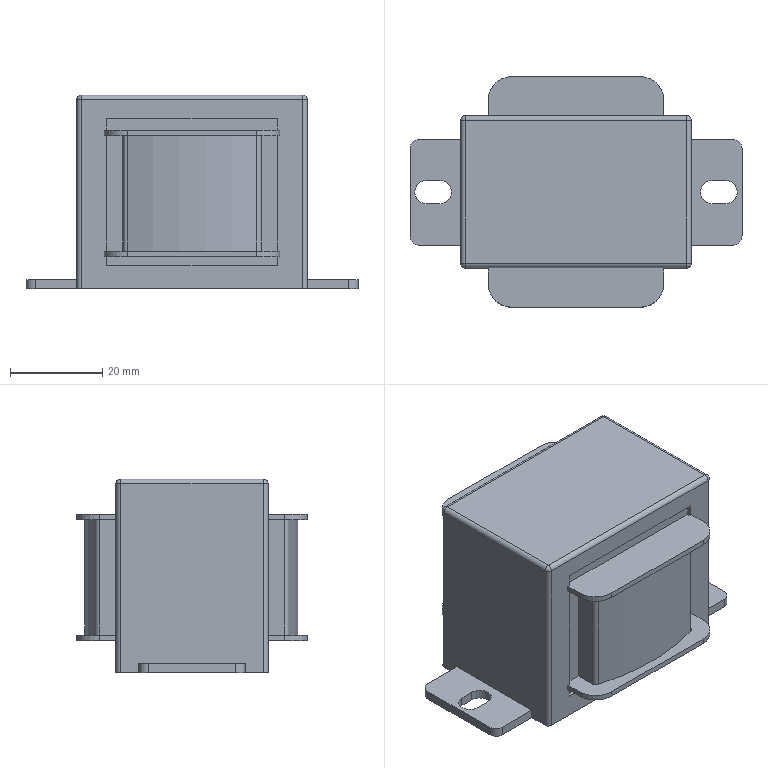Part | STEP file | PN_0019-default | 1 solid | 100 faces | box 72 x 50 x 42 mm | volume 79868 mm3 | plane 66 | cylinder 30 | sphere 4 | commonest cylinder face diameters 2 x12 10 x8 4 x4 5 x4 84.607 x1 96.013 x1